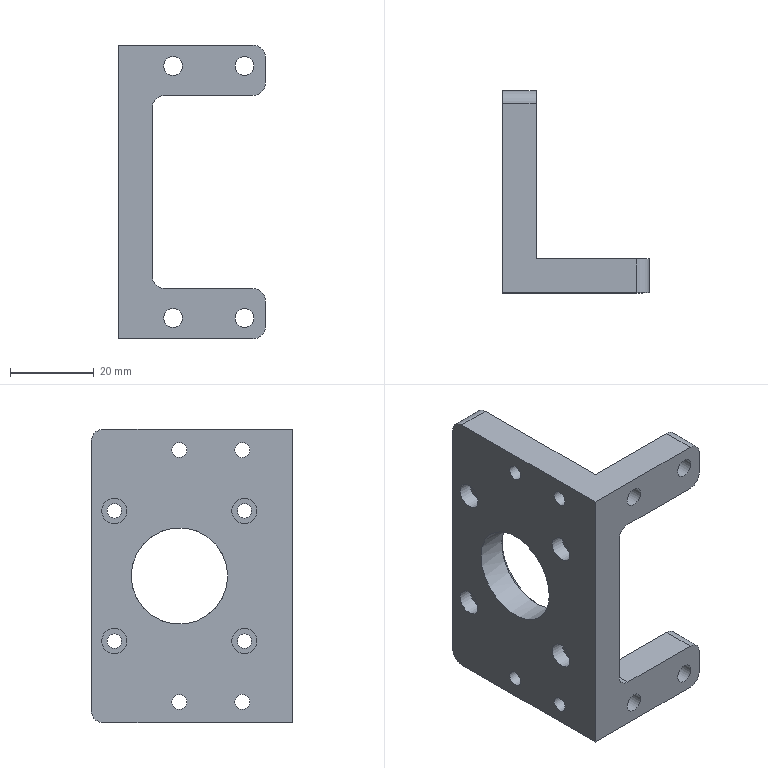Part | 1 solid | 58 faces | box 35 x 48 x 70 mm | volume 26377 mm3 | cylinder 33 | plane 24 | cone 1 | commonest cylinder face diameters 6 x16 3.4 x4 3.6 x4 4.5 x4 8 x4 23 x1
STEP:
#1=CARTESIAN_POINT('',(4.6,12.,68.));
#2=VERTEX_POINT('',#1);
#3=CARTESIAN_POINT('',(4.6,12.,65.));
#4=DIRECTION('',(1.,0.,0.));
#5=DIRECTION('',(0.,0.,1.));
#6=AXIS2_PLACEMENT_3D('',#3,#4,#5);
#7=CIRCLE('',#6,3.);
#8=EDGE_CURVE('',#2,#2,#7,.T.);
#9=ORIENTED_EDGE('',*,*,#8,.T.);
#10=EDGE_LOOP('',(#9));
#11=FACE_BOUND('',#10,.T.);
#12=CARTESIAN_POINT('',(4.6,12.,66.8));
#13=VERTEX_POINT('',#12);
#14=CARTESIAN_POINT('',(4.6,12.,65.));
#15=DIRECTION('',(1.,0.,0.));
#16=DIRECTION('',(0.,0.,1.));
#17=AXIS2_PLACEMENT_3D('',#14,#15,#16);
#18=CIRCLE('',#17,1.8);
#19=EDGE_CURVE('',#13,#13,#18,.T.);
#20=ORIENTED_EDGE('',*,*,#19,.F.);
#21=EDGE_LOOP('',(#20));
#22=FACE_BOUND('',#21,.T.);
#23=CARTESIAN_POINT('',(4.6,13.8,5.));
#24=DIRECTION('',(-1.,0.,0.));
#25=DIRECTION('',(0.,0.,1.));
#26=AXIS2_PLACEMENT_3D('',#23,#24,#25);
#27=PLANE('',#26);
#28=ADVANCED_FACE('',(#11,#22),#27,.F.);
#29=CARTESIAN_POINT('',(4.6,12.,2.));
#30=VERTEX_POINT('',#29);
#31=CARTESIAN_POINT('',(4.6,12.,5.));
#32=DIRECTION('',(1.,0.,0.));
#33=DIRECTION('',(0.,0.,-1.));
#34=AXIS2_PLACEMENT_3D('',#31,#32,#33);
#35=CIRCLE('',#34,3.);
#36=EDGE_CURVE('',#30,#30,#35,.T.);
#37=ORIENTED_EDGE('',*,*,#36,.T.);
#38=EDGE_LOOP('',(#37));
#39=FACE_BOUND('',#38,.T.);
#40=CARTESIAN_POINT('',(4.6,12.,3.2));
#41=VERTEX_POINT('',#40);
#42=CARTESIAN_POINT('',(4.6,12.,5.));
#43=DIRECTION('',(1.,0.,0.));
#44=DIRECTION('',(0.,0.,-1.));
#45=AXIS2_PLACEMENT_3D('',#42,#43,#44);
#46=CIRCLE('',#45,1.8);
#47=EDGE_CURVE('',#41,#41,#46,.T.);
#48=ORIENTED_EDGE('',*,*,#47,.F.);
#49=EDGE_LOOP('',(#48));
#50=FACE_BOUND('',#49,.T.);
#51=CARTESIAN_POINT('',(4.6,13.8,5.));
#52=DIRECTION('',(-1.,0.,0.));
#53=DIRECTION('',(0.,0.,1.));
#54=AXIS2_PLACEMENT_3D('',#51,#52,#53);
#55=PLANE('',#54);
#56=ADVANCED_FACE('',(#39,#50),#55,.F.);
#57=CARTESIAN_POINT('',(4.6,27.,68.));
#58=VERTEX_POINT('',#57);
#59=CARTESIAN_POINT('',(4.6,27.,65.));
#60=DIRECTION('',(1.,0.,0.));
#61=DIRECTION('',(0.,0.,1.));
#62=AXIS2_PLACEMENT_3D('',#59,#60,#61);
#63=CIRCLE('',#62,3.);
#64=EDGE_CURVE('',#58,#58,#63,.T.);
#65=ORIENTED_EDGE('',*,*,#64,.T.);
#66=EDGE_LOOP('',(#65));
#67=FACE_BOUND('',#66,.T.);
#68=CARTESIAN_POINT('',(4.6,27.,66.8));
#69=VERTEX_POINT('',#68);
#70=CARTESIAN_POINT('',(4.6,27.,65.));
#71=DIRECTION('',(1.,0.,0.));
#72=DIRECTION('',(0.,0.,1.));
#73=AXIS2_PLACEMENT_3D('',#70,#71,#72);
#74=CIRCLE('',#73,1.8);
#75=EDGE_CURVE('',#69,#69,#74,.T.);
#76=ORIENTED_EDGE('',*,*,#75,.F.);
#77=EDGE_LOOP('',(#76));
#78=FACE_BOUND('',#77,.T.);
#79=CARTESIAN_POINT('',(4.6,13.8,5.));
#80=DIRECTION('',(-1.,0.,0.));
#81=DIRECTION('',(0.,0.,1.));
#82=AXIS2_PLACEMENT_3D('',#79,#80,#81);
#83=PLANE('',#82);
#84=ADVANCED_FACE('',(#67,#78),#83,.F.);
#85=CARTESIAN_POINT('',(4.6,27.,8.));
#86=VERTEX_POINT('',#85);
#87=CARTESIAN_POINT('',(4.6,27.,5.));
#88=DIRECTION('',(1.,0.,0.));
#89=DIRECTION('',(0.,0.,1.));
#90=AXIS2_PLACEMENT_3D('',#87,#88,#89);
#91=CIRCLE('',#90,3.);
#92=EDGE_CURVE('',#86,#86,#91,.T.);
#93=ORIENTED_EDGE('',*,*,#92,.T.);
#94=EDGE_LOOP('',(#93));
#95=FACE_BOUND('',#94,.T.);
#96=CARTESIAN_POINT('',(4.6,27.,6.8));
#97=VERTEX_POINT('',#96);
#98=CARTESIAN_POINT('',(4.6,27.,5.));
#99=DIRECTION('',(1.,0.,0.));
#100=DIRECTION('',(0.,0.,1.));
#101=AXIS2_PLACEMENT_3D('',#98,#99,#100);
#102=CIRCLE('',#101,1.8);
#103=EDGE_CURVE('',#97,#97,#102,.T.);
#104=ORIENTED_EDGE('',*,*,#103,.F.);
#105=EDGE_LOOP('',(#104));
#106=FACE_BOUND('',#105,.T.);
#107=CARTESIAN_POINT('',(4.6,13.8,5.));
#108=DIRECTION('',(-1.,0.,0.));
#109=DIRECTION('',(0.,0.,1.));
#110=AXIS2_PLACEMENT_3D('',#107,#108,#109);
#111=PLANE('',#110);
#112=ADVANCED_FACE('',(#95,#106),#111,.F.);
#113=CARTESIAN_POINT('',(13.,3.4,69.));
#114=VERTEX_POINT('',#113);
#115=CARTESIAN_POINT('',(13.,3.4,65.));
#116=DIRECTION('',(0.,1.,0.));
#117=DIRECTION('',(0.,0.,1.));
#118=AXIS2_PLACEMENT_3D('',#115,#116,#117);
#119=CIRCLE('',#118,4.);
#120=EDGE_CURVE('',#114,#114,#119,.T.);
#121=ORIENTED_EDGE('',*,*,#120,.T.);
#122=EDGE_LOOP('',(#121));
#123=FACE_BOUND('',#122,.T.);
#124=CARTESIAN_POINT('',(13.,3.4,67.25));
#125=VERTEX_POINT('',#124);
#126=CARTESIAN_POINT('',(13.,3.4,65.));
#127=DIRECTION('',(0.,1.,0.));
#128=DIRECTION('',(0.,0.,1.));
#129=AXIS2_PLACEMENT_3D('',#126,#127,#128);
#130=CIRCLE('',#129,2.25);
#131=EDGE_CURVE('',#125,#125,#130,.T.);
#132=ORIENTED_EDGE('',*,*,#131,.F.);
#133=EDGE_LOOP('',(#132));
#134=FACE_BOUND('',#133,.T.);
#135=CARTESIAN_POINT('',(15.25,3.4,65.));
#136=DIRECTION('',(0.,-1.,0.));
#137=DIRECTION('',(0.,0.,-1.));
#138=AXIS2_PLACEMENT_3D('',#135,#136,#137);
#139=PLANE('',#138);
#140=ADVANCED_FACE('',(#123,#134),#139,.F.);
#141=CARTESIAN_POINT('',(30.,3.4,61.));
#142=VERTEX_POINT('',#141);
#143=CARTESIAN_POINT('',(30.,3.4,65.));
#144=DIRECTION('',(0.,1.,0.));
#145=DIRECTION('',(0.,0.,-1.));
#146=AXIS2_PLACEMENT_3D('',#143,#144,#145);
#147=CIRCLE('',#146,4.);
#148=EDGE_CURVE('',#142,#142,#147,.T.);
#149=ORIENTED_EDGE('',*,*,#148,.T.);
#150=EDGE_LOOP('',(#149));
#151=FACE_BOUND('',#150,.T.);
#152=CARTESIAN_POINT('',(30.,3.4,62.75));
#153=VERTEX_POINT('',#152);
#154=CARTESIAN_POINT('',(30.,3.4,65.));
#155=DIRECTION('',(0.,1.,0.));
#156=DIRECTION('',(0.,0.,-1.));
#157=AXIS2_PLACEMENT_3D('',#154,#155,#156);
#158=CIRCLE('',#157,2.25);
#159=EDGE_CURVE('',#153,#153,#158,.T.);
#160=ORIENTED_EDGE('',*,*,#159,.F.);
#161=EDGE_LOOP('',(#160));
#162=FACE_BOUND('',#161,.T.);
#163=CARTESIAN_POINT('',(15.25,3.4,65.));
#164=DIRECTION('',(0.,-1.,0.));
#165=DIRECTION('',(0.,0.,-1.));
#166=AXIS2_PLACEMENT_3D('',#163,#164,#165);
#167=PLANE('',#166);
#168=ADVANCED_FACE('',(#151,#162),#167,.F.);
#169=CARTESIAN_POINT('',(13.,3.4,1.));
#170=VERTEX_POINT('',#169);
#171=CARTESIAN_POINT('',(13.,3.4,5.));
#172=DIRECTION('',(0.,1.,0.));
#173=DIRECTION('',(0.,0.,-1.));
#174=AXIS2_PLACEMENT_3D('',#171,#172,#173);
#175=CIRCLE('',#174,4.);
#176=EDGE_CURVE('',#170,#170,#175,.T.);
#177=ORIENTED_EDGE('',*,*,#176,.T.);
#178=EDGE_LOOP('',(#177));
#179=FACE_BOUND('',#178,.T.);
#180=CARTESIAN_POINT('',(13.,3.4,2.75));
#181=VERTEX_POINT('',#180);
#182=CARTESIAN_POINT('',(13.,3.4,5.));
#183=DIRECTION('',(0.,1.,0.));
#184=DIRECTION('',(0.,0.,-1.));
#185=AXIS2_PLACEMENT_3D('',#182,#183,#184);
#186=CIRCLE('',#185,2.25);
#187=EDGE_CURVE('',#181,#181,#186,.T.);
#188=ORIENTED_EDGE('',*,*,#187,.F.);
#189=EDGE_LOOP('',(#188));
#190=FACE_BOUND('',#189,.T.);
#191=CARTESIAN_POINT('',(15.25,3.4,65.));
#192=DIRECTION('',(0.,-1.,0.));
#193=DIRECTION('',(0.,0.,-1.));
#194=AXIS2_PLACEMENT_3D('',#191,#192,#193);
#195=PLANE('',#194);
#196=ADVANCED_FACE('',(#179,#190),#195,.F.);
#197=CARTESIAN_POINT('',(30.,3.4,1.));
#198=VERTEX_POINT('',#197);
#199=CARTESIAN_POINT('',(30.,3.4,5.));
#200=DIRECTION('',(0.,1.,0.));
#201=DIRECTION('',(0.,0.,-1.));
#202=AXIS2_PLACEMENT_3D('',#199,#200,#201);
#203=CIRCLE('',#202,4.);
#204=EDGE_CURVE('',#198,#198,#203,.T.);
#205=ORIENTED_EDGE('',*,*,#204,.T.);
#206=EDGE_LOOP('',(#205));
#207=FACE_BOUND('',#206,.T.);
#208=CARTESIAN_POINT('',(30.,3.4,2.75));
#209=VERTEX_POINT('',#208);
#210=CARTESIAN_POINT('',(30.,3.4,5.));
#211=DIRECTION('',(0.,1.,0.));
#212=DIRECTION('',(0.,0.,-1.));
#213=AXIS2_PLACEMENT_3D('',#210,#211,#212);
#214=CIRCLE('',#213,2.25);
#215=EDGE_CURVE('',#209,#209,#214,.T.);
#216=ORIENTED_EDGE('',*,*,#215,.F.);
#217=EDGE_LOOP('',(#216));
#218=FACE_BOUND('',#217,.T.);
#219=CARTESIAN_POINT('',(15.25,3.4,65.));
#220=DIRECTION('',(0.,-1.,0.));
#221=DIRECTION('',(0.,0.,-1.));
#222=AXIS2_PLACEMENT_3D('',#219,#220,#221);
#223=PLANE('',#222);
#224=ADVANCED_FACE('',(#207,#218),#223,.F.);
#225=CARTESIAN_POINT('',(8.,0.,55.));
#226=VERTEX_POINT('',#225);
#227=CARTESIAN_POINT('',(11.,0.,58.));
#228=VERTEX_POINT('',#227);
#229=CARTESIAN_POINT('',(11.,0.,55.));
#230=DIRECTION('',(0.,1.,0.));
#231=DIRECTION('',(0.,0.,1.));
#232=AXIS2_PLACEMENT_3D('',#229,#230,#231);
#233=CIRCLE('',#232,3.);
#234=EDGE_CURVE('',#226,#228,#233,.T.);
#235=ORIENTED_EDGE('',*,*,#234,.F.);
#236=CARTESIAN_POINT('',(8.,8.,55.));
#237=VERTEX_POINT('',#236);
#238=CARTESIAN_POINT('',(8.,0.,55.));
#239=DIRECTION('',(0.,-1.,0.));
#240=VECTOR('',#239,1000.);
#241=LINE('',#238,#240);
#242=EDGE_CURVE('',#237,#226,#241,.T.);
#243=ORIENTED_EDGE('',*,*,#242,.F.);
#244=CARTESIAN_POINT('',(11.,8.,58.));
#245=VERTEX_POINT('',#244);
#246=CARTESIAN_POINT('',(11.,8.,55.));
#247=DIRECTION('',(0.,-1.,0.));
#248=DIRECTION('',(1.,0.,0.));
#249=AXIS2_PLACEMENT_3D('',#246,#247,#248);
#250=CIRCLE('',#249,3.);
#251=EDGE_CURVE('',#245,#237,#250,.T.);
#252=ORIENTED_EDGE('',*,*,#251,.F.);
#253=CARTESIAN_POINT('',(11.,8.,58.));
#254=DIRECTION('',(0.,1.,0.));
#255=VECTOR('',#254,1000.);
#256=LINE('',#253,#255);
#257=EDGE_CURVE('',#228,#245,#256,.T.);
#258=ORIENTED_EDGE('',*,*,#257,.F.);
#259=EDGE_LOOP('',(#235,#243,#252,#258));
#260=FACE_BOUND('',#259,.T.);
#261=CARTESIAN_POINT('',(11.,-2.,55.));
#262=DIRECTION('',(0.,-1.,0.));
#263=DIRECTION('',(0.,0.,-1.));
#264=AXIS2_PLACEMENT_3D('',#261,#262,#263);
#265=CYLINDRICAL_SURFACE('',#264,3.);
#266=ADVANCED_FACE('',(#260),#265,.F.);
#267=CARTESIAN_POINT('',(11.,0.,12.));
#268=VERTEX_POINT('',#267);
#269=CARTESIAN_POINT('',(8.,0.,15.));
#270=VERTEX_POINT('',#269);
#271=CARTESIAN_POINT('',(11.,0.,15.));
#272=DIRECTION('',(0.,1.,0.));
#273=DIRECTION('',(0.,0.,1.));
#274=AXIS2_PLACEMENT_3D('',#271,#272,#273);
#275=CIRCLE('',#274,3.);
#276=EDGE_CURVE('',#268,#270,#275,.T.);
#277=ORIENTED_EDGE('',*,*,#276,.F.);
#278=CARTESIAN_POINT('',(11.,8.,12.));
#279=VERTEX_POINT('',#278);
#280=CARTESIAN_POINT('',(11.,0.,12.));
#281=DIRECTION('',(0.,-1.,0.));
#282=VECTOR('',#281,1000.);
#283=LINE('',#280,#282);
#284=EDGE_CURVE('',#279,#268,#283,.T.);
#285=ORIENTED_EDGE('',*,*,#284,.F.);
#286=CARTESIAN_POINT('',(8.,8.,15.));
#287=VERTEX_POINT('',#286);
#288=CARTESIAN_POINT('',(11.,8.,15.));
#289=DIRECTION('',(0.,-1.,0.));
#290=DIRECTION('',(1.,0.,0.));
#291=AXIS2_PLACEMENT_3D('',#288,#289,#290);
#292=CIRCLE('',#291,3.);
#293=EDGE_CURVE('',#287,#279,#292,.T.);
#294=ORIENTED_EDGE('',*,*,#293,.F.);
#295=CARTESIAN_POINT('',(8.,8.,15.));
#296=DIRECTION('',(0.,1.,0.));
#297=VECTOR('',#296,1000.);
#298=LINE('',#295,#297);
#299=EDGE_CURVE('',#270,#287,#298,.T.);
#300=ORIENTED_EDGE('',*,*,#299,.F.);
#301=EDGE_LOOP('',(#277,#285,#294,#300));
#302=FACE_BOUND('',#301,.T.);
#303=CARTESIAN_POINT('',(11.,8.,15.));
#304=DIRECTION('',(0.,-1.,0.));
#305=DIRECTION('',(0.,0.,-1.));
#306=AXIS2_PLACEMENT_3D('',#303,#304,#305);
#307=CYLINDRICAL_SURFACE('',#306,3.);
#308=ADVANCED_FACE('',(#302),#307,.F.);
#309=CARTESIAN_POINT('',(35.,0.,9.));
#310=VERTEX_POINT('',#309);
#311=CARTESIAN_POINT('',(32.,0.,12.));
#312=VERTEX_POINT('',#311);
#313=CARTESIAN_POINT('',(32.,0.,9.));
#314=DIRECTION('',(0.,-1.,0.));
#315=DIRECTION('',(0.,0.,1.));
#316=AXIS2_PLACEMENT_3D('',#313,#314,#315);
#317=CIRCLE('',#316,3.);
#318=EDGE_CURVE('',#310,#312,#317,.T.);
#319=ORIENTED_EDGE('',*,*,#318,.F.);
#320=CARTESIAN_POINT('',(35.,8.,9.));
#321=VERTEX_POINT('',#320);
#322=CARTESIAN_POINT('',(35.,0.,9.));
#323=DIRECTION('',(0.,-1.,0.));
#324=VECTOR('',#323,1000.);
#325=LINE('',#322,#324);
#326=EDGE_CURVE('',#321,#310,#325,.T.);
#327=ORIENTED_EDGE('',*,*,#326,.F.);
#328=CARTESIAN_POINT('',(32.,8.,12.));
#329=VERTEX_POINT('',#328);
#330=CARTESIAN_POINT('',(32.,8.,9.));
#331=DIRECTION('',(0.,1.,0.));
#332=DIRECTION('',(1.,0.,0.));
#333=AXIS2_PLACEMENT_3D('',#330,#331,#332);
#334=CIRCLE('',#333,3.);
#335=EDGE_CURVE('',#329,#321,#334,.T.);
#336=ORIENTED_EDGE('',*,*,#335,.F.);
#337=CARTESIAN_POINT('',(32.,-2.,12.));
#338=DIRECTION('',(0.,1.,0.));
#339=VECTOR('',#338,1000.);
#340=LINE('',#337,#339);
#341=EDGE_CURVE('',#312,#329,#340,.T.);
#342=ORIENTED_EDGE('',*,*,#341,.F.);
#343=EDGE_LOOP('',(#319,#327,#336,#342));
#344=FACE_BOUND('',#343,.T.);
#345=CARTESIAN_POINT('',(32.,-2.,9.));
#346=DIRECTION('',(0.,1.,0.));
#347=DIRECTION('',(0.,0.,1.));
#348=AXIS2_PLACEMENT_3D('',#345,#346,#347);
#349=CYLINDRICAL_SURFACE('',#348,3.);
#350=ADVANCED_FACE('',(#344),#349,.T.);
#351=CARTESIAN_POINT('',(32.,0.,0.));
#352=VERTEX_POINT('',#351);
#353=CARTESIAN_POINT('',(35.,0.,3.));
#354=VERTEX_POINT('',#353);
#355=CARTESIAN_POINT('',(32.,0.,3.));
#356=DIRECTION('',(0.,-1.,0.));
#357=DIRECTION('',(0.,0.,1.));
#358=AXIS2_PLACEMENT_3D('',#355,#356,#357);
#359=CIRCLE('',#358,3.);
#360=EDGE_CURVE('',#352,#354,#359,.T.);
#361=ORIENTED_EDGE('',*,*,#360,.F.);
#362=CARTESIAN_POINT('',(32.,8.,0.));
#363=VERTEX_POINT('',#362);
#364=CARTESIAN_POINT('',(32.,0.,0.));
#365=DIRECTION('',(0.,-1.,0.));
#366=VECTOR('',#365,1000.);
#367=LINE('',#364,#366);
#368=EDGE_CURVE('',#363,#352,#367,.T.);
#369=ORIENTED_EDGE('',*,*,#368,.F.);
#370=CARTESIAN_POINT('',(35.,8.,3.));
#371=VERTEX_POINT('',#370);
#372=CARTESIAN_POINT('',(32.,8.,3.));
#373=DIRECTION('',(0.,1.,0.));
#374=DIRECTION('',(1.,0.,0.));
#375=AXIS2_PLACEMENT_3D('',#372,#373,#374);
#376=CIRCLE('',#375,3.);
#377=EDGE_CURVE('',#371,#363,#376,.T.);
#378=ORIENTED_EDGE('',*,*,#377,.F.);
#379=CARTESIAN_POINT('',(35.,0.,3.));
#380=DIRECTION('',(0.,1.,0.));
#381=VECTOR('',#380,1000.);
#382=LINE('',#379,#381);
#383=EDGE_CURVE('',#354,#371,#382,.T.);
#384=ORIENTED_EDGE('',*,*,#383,.F.);
#385=EDGE_LOOP('',(#361,#369,#378,#384));
#386=FACE_BOUND('',#385,.T.);
#387=CARTESIAN_POINT('',(32.,0.,3.));
#388=DIRECTION('',(0.,1.,0.));
#389=DIRECTION('',(0.,0.,1.));
#390=AXIS2_PLACEMENT_3D('',#387,#388,#389);
#391=CYLINDRICAL_SURFACE('',#390,3.);
#392=ADVANCED_FACE('',(#386),#391,.T.);
#393=CARTESIAN_POINT('',(32.,0.,58.));
#394=VERTEX_POINT('',#393);
#395=CARTESIAN_POINT('',(35.,0.,61.));
#396=VERTEX_POINT('',#395);
#397=CARTESIAN_POINT('',(32.,0.,61.));
#398=DIRECTION('',(0.,-1.,0.));
#399=DIRECTION('',(0.,0.,1.));
#400=AXIS2_PLACEMENT_3D('',#397,#398,#399);
#401=CIRCLE('',#400,3.);
#402=EDGE_CURVE('',#394,#396,#401,.T.);
#403=ORIENTED_EDGE('',*,*,#402,.F.);
#404=CARTESIAN_POINT('',(32.,8.,58.));
#405=VERTEX_POINT('',#404);
#406=CARTESIAN_POINT('',(32.,-2.,58.));
#407=DIRECTION('',(0.,-1.,0.));
#408=VECTOR('',#407,1000.);
#409=LINE('',#406,#408);
#410=EDGE_CURVE('',#405,#394,#409,.T.);
#411=ORIENTED_EDGE('',*,*,#410,.F.);
#412=CARTESIAN_POINT('',(35.,8.,61.));
#413=VERTEX_POINT('',#412);
#414=CARTESIAN_POINT('',(32.,8.,61.));
#415=DIRECTION('',(0.,1.,0.));
#416=DIRECTION('',(1.,0.,0.));
#417=AXIS2_PLACEMENT_3D('',#414,#415,#416);
#418=CIRCLE('',#417,3.);
#419=EDGE_CURVE('',#413,#405,#418,.T.);
#420=ORIENTED_EDGE('',*,*,#419,.F.);
#421=CARTESIAN_POINT('',(35.,0.,61.));
#422=DIRECTION('',(0.,1.,0.));
#423=VECTOR('',#422,1000.);
#424=LINE('',#421,#423);
#425=EDGE_CURVE('',#396,#413,#424,.T.);
#426=ORIENTED_EDGE('',*,*,#425,.F.);
#427=EDGE_LOOP('',(#403,#411,#420,#426));
#428=FACE_BOUND('',#427,.T.);
#429=CARTESIAN_POINT('',(32.,0.,61.));
#430=DIRECTION('',(0.,1.,0.));
#431=DIRECTION('',(0.,0.,1.));
#432=AXIS2_PLACEMENT_3D('',#429,#430,#431);
#433=CYLINDRICAL_SURFACE('',#432,3.);
#434=ADVANCED_FACE('',(#428),#433,.T.);
#435=CARTESIAN_POINT('',(35.,0.,67.));
#436=VERTEX_POINT('',#435);
#437=CARTESIAN_POINT('',(32.,0.,70.));
#438=VERTEX_POINT('',#437);
#439=CARTESIAN_POINT('',(32.,0.,67.));
#440=DIRECTION('',(0.,-1.,0.));
#441=DIRECTION('',(0.,0.,1.));
#442=AXIS2_PLACEMENT_3D('',#439,#440,#441);
#443=CIRCLE('',#442,3.);
#444=EDGE_CURVE('',#436,#438,#443,.T.);
#445=ORIENTED_EDGE('',*,*,#444,.F.);
#446=CARTESIAN_POINT('',(35.,8.,67.));
#447=VERTEX_POINT('',#446);
#448=CARTESIAN_POINT('',(35.,0.,67.));
#449=DIRECTION('',(0.,-1.,0.));
#450=VECTOR('',#449,1000.);
#451=LINE('',#448,#450);
#452=EDGE_CURVE('',#447,#436,#451,.T.);
#453=ORIENTED_EDGE('',*,*,#452,.F.);
#454=CARTESIAN_POINT('',(32.,8.,70.));
#455=VERTEX_POINT('',#454);
#456=CARTESIAN_POINT('',(32.,8.,67.));
#457=DIRECTION('',(0.,1.,0.));
#458=DIRECTION('',(1.,0.,0.));
#459=AXIS2_PLACEMENT_3D('',#456,#457,#458);
#460=CIRCLE('',#459,3.);
#461=EDGE_CURVE('',#455,#447,#460,.T.);
#462=ORIENTED_EDGE('',*,*,#461,.F.);
#463=CARTESIAN_POINT('',(32.,8.,70.));
#464=DIRECTION('',(0.,1.,0.));
#465=VECTOR('',#464,1000.);
#466=LINE('',#463,#465);
#467=EDGE_CURVE('',#438,#455,#466,.T.);
#468=ORIENTED_EDGE('',*,*,#467,.F.);
#469=EDGE_LOOP('',(#445,#453,#462,#468));
#470=FACE_BOUND('',#469,.T.);
#471=CARTESIAN_POINT('',(32.,0.,67.));
#472=DIRECTION('',(0.,-1.,0.));
#473=DIRECTION('',(0.,0.,-1.));
#474=AXIS2_PLACEMENT_3D('',#471,#472,#473);
#475=CYLINDRICAL_SURFACE('',#474,3.);
#476=ADVANCED_FACE('',(#470),#475,.T.);
#477=CARTESIAN_POINT('',(8.,48.,67.));
#478=VERTEX_POINT('',#477);
#479=CARTESIAN_POINT('',(8.,45.,70.));
#480=VERTEX_POINT('',#479);
#481=CARTESIAN_POINT('',(8.,45.,67.));
#482=DIRECTION('',(1.,0.,0.));
#483=DIRECTION('',(0.,0.,1.));
#484=AXIS2_PLACEMENT_3D('',#481,#482,#483);
#485=CIRCLE('',#484,3.);
#486=EDGE_CURVE('',#478,#480,#485,.T.);
#487=ORIENTED_EDGE('',*,*,#486,.F.);
#488=CARTESIAN_POINT('',(0.,48.,67.));
#489=VERTEX_POINT('',#488);
#490=CARTESIAN_POINT('',(8.,48.,67.));
#491=DIRECTION('',(1.,0.,0.));
#492=VECTOR('',#491,1000.);
#493=LINE('',#490,#492);
#494=EDGE_CURVE('',#489,#478,#493,.T.);
#495=ORIENTED_EDGE('',*,*,#494,.F.);
#496=CARTESIAN_POINT('',(0.,45.,70.));
#497=VERTEX_POINT('',#496);
#498=CARTESIAN_POINT('',(0.,45.,67.));
#499=DIRECTION('',(-1.,0.,0.));
#500=DIRECTION('',(0.,0.,-1.));
#501=AXIS2_PLACEMENT_3D('',#498,#499,#500);
#502=CIRCLE('',#501,3.);
#503=EDGE_CURVE('',#497,#489,#502,.T.);
#504=ORIENTED_EDGE('',*,*,#503,.F.);
#505=CARTESIAN_POINT('',(0.,45.,70.));
#506=DIRECTION('',(-1.,0.,0.));
#507=VECTOR('',#506,1000.);
#508=LINE('',#505,#507);
#509=EDGE_CURVE('',#480,#497,#508,.T.);
#510=ORIENTED_EDGE('',*,*,#509,.F.);
#511=EDGE_LOOP('',(#487,#495,#504,#510));
#512=FACE_BOUND('',#511,.T.);
#513=CARTESIAN_POINT('',(0.,45.,67.));
#514=DIRECTION('',(1.,0.,0.));
#515=DIRECTION('',(0.,0.,-1.));
#516=AXIS2_PLACEMENT_3D('',#513,#514,#515);
#517=CYLINDRICAL_SURFACE('',#516,3.);
#518=ADVANCED_FACE('',(#512),#517,.T.);
#519=CARTESIAN_POINT('',(8.,45.,0.));
#520=VERTEX_POINT('',#519);
#521=CARTESIAN_POINT('',(8.,48.,3.));
#522=VERTEX_POINT('',#521);
#523=CARTESIAN_POINT('',(8.,45.,3.));
#524=DIRECTION('',(1.,0.,0.));
#525=DIRECTION('',(0.,0.,1.));
#526=AXIS2_PLACEMENT_3D('',#523,#524,#525);
#527=CIRCLE('',#526,3.);
#528=EDGE_CURVE('',#520,#522,#527,.T.);
#529=ORIENTED_EDGE('',*,*,#528,.F.);
#530=CARTESIAN_POINT('',(0.,45.,0.));
#531=VERTEX_POINT('',#530);
#532=CARTESIAN_POINT('',(0.,45.,0.));
#533=DIRECTION('',(1.,0.,0.));
#534=VECTOR('',#533,1000.);
#535=LINE('',#532,#534);
#536=EDGE_CURVE('',#531,#520,#535,.T.);
#537=ORIENTED_EDGE('',*,*,#536,.F.);
#538=CARTESIAN_POINT('',(0.,48.,3.));
#539=VERTEX_POINT('',#538);
#540=CARTESIAN_POINT('',(0.,45.,3.));
#541=DIRECTION('',(-1.,0.,0.));
#542=DIRECTION('',(0.,0.,-1.));
#543=AXIS2_PLACEMENT_3D('',#540,#541,#542);
#544=CIRCLE('',#543,3.);
#545=EDGE_CURVE('',#539,#531,#544,.T.);
#546=ORIENTED_EDGE('',*,*,#545,.F.);
#547=CARTESIAN_POINT('',(8.,48.,3.));
#548=DIRECTION('',(-1.,0.,0.));
#549=VECTOR('',#548,1000.);
#550=LINE('',#547,#549);
#551=EDGE_CURVE('',#522,#539,#550,.T.);
#552=ORIENTED_EDGE('',*,*,#551,.F.);
#553=EDGE_LOOP('',(#529,#537,#546,#552));
#554=FACE_BOUND('',#553,.T.);
#555=CARTESIAN_POINT('',(8.,45.,3.));
#556=DIRECTION('',(-1.,0.,0.));
#557=DIRECTION('',(0.,0.,1.));
#558=AXIS2_PLACEMENT_3D('',#555,#556,#557);
#559=CYLINDRICAL_SURFACE('',#558,3.);
#560=ADVANCED_FACE('',(#554),#559,.T.);
#561=CARTESIAN_POINT('',(8.,8.,58.));
#562=DIRECTION('',(1.,0.,0.));
#563=VECTOR('',#562,1000.);
#564=LINE('',#561,#563);
#565=EDGE_CURVE('',#245,#405,#564,.T.);
#566=ORIENTED_EDGE('',*,*,#565,.T.);
#567=ORIENTED_EDGE('',*,*,#410,.T.);
#568=CARTESIAN_POINT('',(0.,0.,58.));
#569=DIRECTION('',(1.,0.,0.));
#570=VECTOR('',#569,1000.);
#571=LINE('',#568,#570);
#572=EDGE_CURVE('',#228,#394,#571,.T.);
#573=ORIENTED_EDGE('',*,*,#572,.F.);
#574=ORIENTED_EDGE('',*,*,#257,.T.);
#575=EDGE_LOOP('',(#566,#567,#573,#574));
#576=FACE_BOUND('',#575,.T.);
#577=CARTESIAN_POINT('',(8.,-2.,58.));
#578=DIRECTION('',(0.,0.,1.));
#579=DIRECTION('',(1.,0.,0.));
#580=AXIS2_PLACEMENT_3D('',#577,#578,#579);
#581=PLANE('',#580);
#582=ADVANCED_FACE('',(#576),#581,.F.);
#583=CARTESIAN_POINT('',(0.,0.,12.));
#584=DIRECTION('',(-1.,0.,0.));
#585=VECTOR('',#584,1000.);
#586=LINE('',#583,#585);
#587=EDGE_CURVE('',#312,#268,#586,.T.);
#588=ORIENTED_EDGE('',*,*,#587,.F.);
#589=ORIENTED_EDGE('',*,*,#341,.T.);
#590=CARTESIAN_POINT('',(8.,8.,12.));
#591=DIRECTION('',(-1.,0.,0.));
#592=VECTOR('',#591,1000.);
#593=LINE('',#590,#592);
#594=EDGE_CURVE('',#329,#279,#593,.T.);
#595=ORIENTED_EDGE('',*,*,#594,.T.);
#596=ORIENTED_EDGE('',*,*,#284,.T.);
#597=EDGE_LOOP('',(#588,#589,#595,#596));
#598=FACE_BOUND('',#597,.T.);
#599=CARTESIAN_POINT('',(8.,-2.,12.));
#600=DIRECTION('',(0.,0.,-1.));
#601=DIRECTION('',(-1.,0.,0.));
#602=AXIS2_PLACEMENT_3D('',#599,#600,#601);
#603=PLANE('',#602);
#604=ADVANCED_FACE('',(#598),#603,.F.);
#605=CARTESIAN_POINT('',(3.4,42.5,53.5));
#606=VERTEX_POINT('',#605);
#607=CARTESIAN_POINT('',(3.4,42.5,50.5));
#608=DIRECTION('',(-1.,0.,0.));
#609=DIRECTION('',(0.,0.,1.));
#610=AXIS2_PLACEMENT_3D('',#607,#608,#609);
#611=CIRCLE('',#610,3.);
#612=EDGE_CURVE('',#606,#606,#611,.T.);
#613=ORIENTED_EDGE('',*,*,#612,.T.);
#614=EDGE_LOOP('',(#613));
#615=FACE_BOUND('',#614,.T.);
#616=CARTESIAN_POINT('',(3.4,42.5,52.2));
#617=VERTEX_POINT('',#616);
#618=CARTESIAN_POINT('',(3.4,42.5,50.5));
#619=DIRECTION('',(-1.,0.,0.));
#620=DIRECTION('',(0.,0.,1.));
#621=AXIS2_PLACEMENT_3D('',#618,#619,#620);
#622=CIRCLE('',#621,1.7);
#623=EDGE_CURVE('',#617,#617,#622,.T.);
#624=ORIENTED_EDGE('',*,*,#623,.F.);
#625=EDGE_LOOP('',(#624));
#626=FACE_BOUND('',#625,.T.);
#627=CARTESIAN_POINT('',(3.4,44.2,50.5));
#628=DIRECTION('',(1.,0.,0.));
#629=DIRECTION('',(0.,0.,-1.));
#630=AXIS2_PLACEMENT_3D('',#627,#628,#629);
#631=PLANE('',#630);
#632=ADVANCED_FACE('',(#615,#626),#631,.F.);
#633=CARTESIAN_POINT('',(3.4,11.5,16.5));
#634=VERTEX_POINT('',#633);
#635=CARTESIAN_POINT('',(3.4,11.5,19.5));
#636=DIRECTION('',(-1.,0.,0.));
#637=DIRECTION('',(0.,0.,-1.));
#638=AXIS2_PLACEMENT_3D('',#635,#636,#637);
#639=CIRCLE('',#638,3.);
#640=EDGE_CURVE('',#634,#634,#639,.T.);
#641=ORIENTED_EDGE('',*,*,#640,.T.);
#642=EDGE_LOOP('',(#641));
#643=FACE_BOUND('',#642,.T.);
#644=CARTESIAN_POINT('',(3.4,11.5,17.8));
#645=VERTEX_POINT('',#644);
#646=CARTESIAN_POINT('',(3.4,11.5,19.5));
#647=DIRECTION('',(-1.,0.,0.));
#648=DIRECTION('',(0.,0.,-1.));
#649=AXIS2_PLACEMENT_3D('',#646,#647,#648);
#650=CIRCLE('',#649,1.7);
#651=EDGE_CURVE('',#645,#645,#650,.T.);
#652=ORIENTED_EDGE('',*,*,#651,.F.);
#653=EDGE_LOOP('',(#652));
#654=FACE_BOUND('',#653,.T.);
#655=CARTESIAN_POINT('',(3.4,44.2,50.5));
#656=DIRECTION('',(1.,0.,0.));
#657=DIRECTION('',(0.,0.,-1.));
#658=AXIS2_PLACEMENT_3D('',#655,#656,#657);
#659=PLANE('',#658);
#660=ADVANCED_FACE('',(#643,#654),#659,.F.);
#661=CARTESIAN_POINT('',(3.4,42.5,16.5));
#662=VERTEX_POINT('',#661);
#663=CARTESIAN_POINT('',(3.4,42.5,19.5));
#664=DIRECTION('',(-1.,0.,0.));
#665=DIRECTION('',(0.,0.,-1.));
#666=AXIS2_PLACEMENT_3D('',#663,#664,#665);
#667=CIRCLE('',#666,3.);
#668=EDGE_CURVE('',#662,#662,#667,.T.);
#669=ORIENTED_EDGE('',*,*,#668,.T.);
#670=EDGE_LOOP('',(#669));
#671=FACE_BOUND('',#670,.T.);
#672=CARTESIAN_POINT('',(3.4,42.5,17.8));
#673=VERTEX_POINT('',#672);
#674=CARTESIAN_POINT('',(3.4,42.5,19.5));
#675=DIRECTION('',(-1.,0.,0.));
#676=DIRECTION('',(0.,0.,-1.));
#677=AXIS2_PLACEMENT_3D('',#674,#675,#676);
#678=CIRCLE('',#677,1.7);
#679=EDGE_CURVE('',#673,#673,#678,.T.);
#680=ORIENTED_EDGE('',*,*,#679,.F.);
#681=EDGE_LOOP('',(#680));
#682=FACE_BOUND('',#681,.T.);
#683=CARTESIAN_POINT('',(3.4,44.2,50.5));
#684=DIRECTION('',(1.,0.,0.));
#685=DIRECTION('',(0.,0.,-1.));
#686=AXIS2_PLACEMENT_3D('',#683,#684,#685);
#687=PLANE('',#686);
#688=ADVANCED_FACE('',(#671,#682),#687,.F.);
#689=CARTESIAN_POINT('',(3.4,11.5,47.5));
#690=VERTEX_POINT('',#689);
#691=CARTESIAN_POINT('',(3.4,11.5,50.5));
#692=DIRECTION('',(-1.,0.,0.));
#693=DIRECTION('',(0.,0.,-1.));
#694=AXIS2_PLACEMENT_3D('',#691,#692,#693);
#695=CIRCLE('',#694,3.);
#696=EDGE_CURVE('',#690,#690,#695,.T.);
#697=ORIENTED_EDGE('',*,*,#696,.T.);
#698=EDGE_LOOP('',(#697));
#699=FACE_BOUND('',#698,.T.);
#700=CARTESIAN_POINT('',(3.4,11.5,48.8));
#701=VERTEX_POINT('',#700);
#702=CARTESIAN_POINT('',(3.4,11.5,50.5));
#703=DIRECTION('',(-1.,0.,0.));
#704=DIRECTION('',(0.,0.,-1.));
#705=AXIS2_PLACEMENT_3D('',#702,#703,#704);
#706=CIRCLE('',#705,1.7);
#707=EDGE_CURVE('',#701,#701,#706,.T.);
#708=ORIENTED_EDGE('',*,*,#707,.F.);
#709=EDGE_LOOP('',(#708));
#710=FACE_BOUND('',#709,.T.);
#711=CARTESIAN_POINT('',(3.4,44.2,50.5));
#712=DIRECTION('',(1.,0.,0.));
#713=DIRECTION('',(0.,0.,-1.));
#714=AXIS2_PLACEMENT_3D('',#711,#712,#713);
#715=PLANE('',#714);
#716=ADVANCED_FACE('',(#699,#710),#715,.F.);
#717=CARTESIAN_POINT('',(0.,0.,0.));
#718=VERTEX_POINT('',#717);
#719=CARTESIAN_POINT('',(0.,48.,0.));
#720=DIRECTION('',(0.,-1.,0.));
#721=VECTOR('',#720,1000.);
#722=LINE('',#719,#721);
#723=EDGE_CURVE('',#531,#718,#722,.T.);
#724=ORIENTED_EDGE('',*,*,#723,.F.);
#725=ORIENTED_EDGE('',*,*,#536,.T.);
#726=CARTESIAN_POINT('',(8.,8.,0.));
#727=VERTEX_POINT('',#726);
#728=CARTESIAN_POINT('',(8.,8.,0.));
#729=DIRECTION('',(0.,1.,0.));
#730=VECTOR('',#729,1000.);
#731=LINE('',#728,#730);
#732=EDGE_CURVE('',#727,#520,#731,.T.);
#733=ORIENTED_EDGE('',*,*,#732,.F.);
#734=CARTESIAN_POINT('',(35.,8.,0.));
#735=DIRECTION('',(-1.,0.,0.));
#736=VECTOR('',#735,1000.);
#737=LINE('',#734,#736);
#738=EDGE_CURVE('',#363,#727,#737,.T.);
#739=ORIENTED_EDGE('',*,*,#738,.F.);
#740=ORIENTED_EDGE('',*,*,#368,.T.);
#741=CARTESIAN_POINT('',(0.,0.,0.));
#742=DIRECTION('',(1.,0.,0.));
#743=VECTOR('',#742,1000.);
#744=LINE('',#741,#743);
#745=EDGE_CURVE('',#718,#352,#744,.T.);
#746=ORIENTED_EDGE('',*,*,#745,.F.);
#747=EDGE_LOOP('',(#724,#725,#733,#739,#740,#746));
#748=FACE_BOUND('',#747,.T.);
#749=CARTESIAN_POINT('',(0.,0.,0.));
#750=DIRECTION('',(0.,0.,1.));
#751=DIRECTION('',(1.,0.,0.));
#752=AXIS2_PLACEMENT_3D('',#749,#750,#751);
#753=PLANE('',#752);
#754=ADVANCED_FACE('',(#748),#753,.F.);
#755=CARTESIAN_POINT('',(8.,8.,70.));
#756=VERTEX_POINT('',#755);
#757=CARTESIAN_POINT('',(8.,8.,70.));
#758=DIRECTION('',(0.,1.,0.));
#759=VECTOR('',#758,1000.);
#760=LINE('',#757,#759);
#761=EDGE_CURVE('',#756,#480,#760,.T.);
#762=ORIENTED_EDGE('',*,*,#761,.T.);
#763=ORIENTED_EDGE('',*,*,#509,.T.);
#764=CARTESIAN_POINT('',(0.,0.,70.));
#765=VERTEX_POINT('',#764);
#766=CARTESIAN_POINT('',(0.,48.,70.));
#767=DIRECTION('',(0.,-1.,0.));
#768=VECTOR('',#767,1000.);
#769=LINE('',#766,#768);
#770=EDGE_CURVE('',#497,#765,#769,.T.);
#771=ORIENTED_EDGE('',*,*,#770,.T.);
#772=CARTESIAN_POINT('',(0.,0.,70.));
#773=DIRECTION('',(1.,0.,0.));
#774=VECTOR('',#773,1000.);
#775=LINE('',#772,#774);
#776=EDGE_CURVE('',#765,#438,#775,.T.);
#777=ORIENTED_EDGE('',*,*,#776,.T.);
#778=ORIENTED_EDGE('',*,*,#467,.T.);
#779=CARTESIAN_POINT('',(35.,8.,70.));
#780=DIRECTION('',(-1.,0.,0.));
#781=VECTOR('',#780,1000.);
#782=LINE('',#779,#781);
#783=EDGE_CURVE('',#455,#756,#782,.T.);
#784=ORIENTED_EDGE('',*,*,#783,.T.);
#785=EDGE_LOOP('',(#762,#763,#771,#777,#778,#784));
#786=FACE_BOUND('',#785,.T.);
#787=CARTESIAN_POINT('',(0.,0.,70.));
#788=DIRECTION('',(0.,0.,1.));
#789=DIRECTION('',(1.,0.,0.));
#790=AXIS2_PLACEMENT_3D('',#787,#788,#789);
#791=PLANE('',#790);
#792=ADVANCED_FACE('',(#786),#791,.T.);
#793=ORIENTED_EDGE('',*,*,#732,.T.);
#794=ORIENTED_EDGE('',*,*,#528,.T.);
#795=CARTESIAN_POINT('',(8.,48.,70.));
#796=DIRECTION('',(0.,0.,-1.));
#797=VECTOR('',#796,1000.);
#798=LINE('',#795,#797);
#799=EDGE_CURVE('',#478,#522,#798,.T.);
#800=ORIENTED_EDGE('',*,*,#799,.F.);
#801=ORIENTED_EDGE('',*,*,#486,.T.);
#802=ORIENTED_EDGE('',*,*,#761,.F.);
#803=CARTESIAN_POINT('',(8.,8.,70.));
#804=DIRECTION('',(0.,0.,-1.));
#805=VECTOR('',#804,1000.);
#806=LINE('',#803,#805);
#807=EDGE_CURVE('',#756,#237,#806,.T.);
#808=ORIENTED_EDGE('',*,*,#807,.T.);
#809=ORIENTED_EDGE('',*,*,#242,.T.);
#810=CARTESIAN_POINT('',(8.,0.,70.));
#811=DIRECTION('',(0.,0.,1.));
#812=VECTOR('',#811,1000.);
#813=LINE('',#810,#812);
#814=EDGE_CURVE('',#270,#226,#813,.T.);
#815=ORIENTED_EDGE('',*,*,#814,.F.);
#816=ORIENTED_EDGE('',*,*,#299,.T.);
#817=CARTESIAN_POINT('',(8.,8.,70.));
#818=DIRECTION('',(0.,0.,-1.));
#819=VECTOR('',#818,1000.);
#820=LINE('',#817,#819);
#821=EDGE_CURVE('',#287,#727,#820,.T.);
#822=ORIENTED_EDGE('',*,*,#821,.T.);
#823=EDGE_LOOP('',(#793,#794,#800,#801,#802,#808,#809,#815,#816,#822));
#824=FACE_BOUND('',#823,.T.);
#825=CARTESIAN_POINT('',(8.,11.5,52.2));
#826=VERTEX_POINT('',#825);
#827=CARTESIAN_POINT('',(8.,11.5,50.5));
#828=DIRECTION('',(-1.,0.,0.));
#829=DIRECTION('',(0.,0.,1.));
#830=AXIS2_PLACEMENT_3D('',#827,#828,#829);
#831=CIRCLE('',#830,1.7);
#832=EDGE_CURVE('',#826,#826,#831,.T.);
#833=ORIENTED_EDGE('',*,*,#832,.T.);
#834=EDGE_LOOP('',(#833));
#835=FACE_BOUND('',#834,.T.);
#836=CARTESIAN_POINT('',(8.,42.5,21.2));
#837=VERTEX_POINT('',#836);
#838=CARTESIAN_POINT('',(8.,42.5,19.5));
#839=DIRECTION('',(-1.,0.,0.));
#840=DIRECTION('',(0.,0.,1.));
#841=AXIS2_PLACEMENT_3D('',#838,#839,#840);
#842=CIRCLE('',#841,1.7);
#843=EDGE_CURVE('',#837,#837,#842,.T.);
#844=ORIENTED_EDGE('',*,*,#843,.T.);
#845=EDGE_LOOP('',(#844));
#846=FACE_BOUND('',#845,.T.);
#847=CARTESIAN_POINT('',(8.,11.5,21.2));
#848=VERTEX_POINT('',#847);
#849=CARTESIAN_POINT('',(8.,11.5,19.5));
#850=DIRECTION('',(-1.,0.,0.));
#851=DIRECTION('',(0.,0.,1.));
#852=AXIS2_PLACEMENT_3D('',#849,#850,#851);
#853=CIRCLE('',#852,1.7);
#854=EDGE_CURVE('',#848,#848,#853,.T.);
#855=ORIENTED_EDGE('',*,*,#854,.T.);
#856=EDGE_LOOP('',(#855));
#857=FACE_BOUND('',#856,.T.);
#858=CARTESIAN_POINT('',(8.,42.5,52.2));
#859=VERTEX_POINT('',#858);
#860=CARTESIAN_POINT('',(8.,42.5,50.5));
#861=DIRECTION('',(-1.,0.,0.));
#862=DIRECTION('',(0.,0.,1.));
#863=AXIS2_PLACEMENT_3D('',#860,#861,#862);
#864=CIRCLE('',#863,1.7);
#865=EDGE_CURVE('',#859,#859,#864,.T.);
#866=ORIENTED_EDGE('',*,*,#865,.T.);
#867=EDGE_LOOP('',(#866));
#868=FACE_BOUND('',#867,.T.);
#869=CARTESIAN_POINT('',(8.,27.,47.5));
#870=VERTEX_POINT('',#869);
#871=CARTESIAN_POINT('',(8.,27.,35.));
#872=DIRECTION('',(-1.,0.,0.));
#873=DIRECTION('',(0.,0.,1.));
#874=AXIS2_PLACEMENT_3D('',#871,#872,#873);
#875=CIRCLE('',#874,12.5);
#876=EDGE_CURVE('',#870,#870,#875,.T.);
#877=ORIENTED_EDGE('',*,*,#876,.T.);
#878=EDGE_LOOP('',(#877));
#879=FACE_BOUND('',#878,.T.);
#880=CARTESIAN_POINT('',(8.,27.,2.));
#881=VERTEX_POINT('',#880);
#882=CARTESIAN_POINT('',(8.,27.,5.));
#883=DIRECTION('',(1.,0.,0.));
#884=DIRECTION('',(0.,0.,-1.));
#885=AXIS2_PLACEMENT_3D('',#882,#883,#884);
#886=CIRCLE('',#885,3.);
#887=EDGE_CURVE('',#881,#881,#886,.T.);
#888=ORIENTED_EDGE('',*,*,#887,.F.);
#889=EDGE_LOOP('',(#888));
#890=FACE_BOUND('',#889,.T.);
#891=CARTESIAN_POINT('',(8.,27.,62.));
#892=VERTEX_POINT('',#891);
#893=CARTESIAN_POINT('',(8.,27.,65.));
#894=DIRECTION('',(1.,0.,0.));
#895=DIRECTION('',(0.,0.,-1.));
#896=AXIS2_PLACEMENT_3D('',#893,#894,#895);
#897=CIRCLE('',#896,3.);
#898=EDGE_CURVE('',#892,#892,#897,.T.);
#899=ORIENTED_EDGE('',*,*,#898,.F.);
#900=EDGE_LOOP('',(#899));
#901=FACE_BOUND('',#900,.T.);
#902=CARTESIAN_POINT('',(8.,12.,2.));
#903=VERTEX_POINT('',#902);
#904=CARTESIAN_POINT('',(8.,12.,5.));
#905=DIRECTION('',(1.,0.,0.));
#906=DIRECTION('',(0.,0.,-1.));
#907=AXIS2_PLACEMENT_3D('',#904,#905,#906);
#908=CIRCLE('',#907,3.);
#909=EDGE_CURVE('',#903,#903,#908,.T.);
#910=ORIENTED_EDGE('',*,*,#909,.F.);
#911=EDGE_LOOP('',(#910));
#912=FACE_BOUND('',#911,.T.);
#913=CARTESIAN_POINT('',(8.,12.,62.));
#914=VERTEX_POINT('',#913);
#915=CARTESIAN_POINT('',(8.,12.,65.));
#916=DIRECTION('',(1.,0.,0.));
#917=DIRECTION('',(0.,0.,-1.));
#918=AXIS2_PLACEMENT_3D('',#915,#916,#917);
#919=CIRCLE('',#918,3.);
#920=EDGE_CURVE('',#914,#914,#919,.T.);
#921=ORIENTED_EDGE('',*,*,#920,.F.);
#922=EDGE_LOOP('',(#921));
#923=FACE_BOUND('',#922,.T.);
#924=CARTESIAN_POINT('',(8.,8.,70.));
#925=DIRECTION('',(-1.,0.,0.));
#926=DIRECTION('',(0.,0.,1.));
#927=AXIS2_PLACEMENT_3D('',#924,#925,#926);
#928=PLANE('',#927);
#929=ADVANCED_FACE('',(#824,#835,#846,#857,#868,#879,#890,#901,#912,#923),#928,.F.);
#930=ORIENTED_EDGE('',*,*,#783,.F.);
#931=ORIENTED_EDGE('',*,*,#461,.T.);
#932=CARTESIAN_POINT('',(35.,8.,70.));
#933=DIRECTION('',(0.,0.,-1.));
#934=VECTOR('',#933,1000.);
#935=LINE('',#932,#934);
#936=EDGE_CURVE('',#447,#413,#935,.T.);
#937=ORIENTED_EDGE('',*,*,#936,.T.);
#938=ORIENTED_EDGE('',*,*,#419,.T.);
#939=ORIENTED_EDGE('',*,*,#565,.F.);
#940=ORIENTED_EDGE('',*,*,#251,.T.);
#941=ORIENTED_EDGE('',*,*,#807,.F.);
#942=EDGE_LOOP('',(#930,#931,#937,#938,#939,#940,#941));
#943=FACE_BOUND('',#942,.T.);
#944=CARTESIAN_POINT('',(30.,8.,69.));
#945=VERTEX_POINT('',#944);
#946=CARTESIAN_POINT('',(30.,8.,65.));
#947=DIRECTION('',(0.,1.,0.));
#948=DIRECTION('',(0.,0.,1.));
#949=AXIS2_PLACEMENT_3D('',#946,#947,#948);
#950=CIRCLE('',#949,4.);
#951=EDGE_CURVE('',#945,#945,#950,.T.);
#952=ORIENTED_EDGE('',*,*,#951,.F.);
#953=EDGE_LOOP('',(#952));
#954=FACE_BOUND('',#953,.T.);
#955=CARTESIAN_POINT('',(13.,8.,69.));
#956=VERTEX_POINT('',#955);
#957=CARTESIAN_POINT('',(13.,8.,65.));
#958=DIRECTION('',(0.,1.,0.));
#959=DIRECTION('',(0.,0.,1.));
#960=AXIS2_PLACEMENT_3D('',#957,#958,#959);
#961=CIRCLE('',#960,4.);
#962=EDGE_CURVE('',#956,#956,#961,.T.);
#963=ORIENTED_EDGE('',*,*,#962,.F.);
#964=EDGE_LOOP('',(#963));
#965=FACE_BOUND('',#964,.T.);
#966=CARTESIAN_POINT('',(35.,8.,70.));
#967=DIRECTION('',(0.,-1.,0.));
#968=DIRECTION('',(1.,0.,0.));
#969=AXIS2_PLACEMENT_3D('',#966,#967,#968);
#970=PLANE('',#969);
#971=ADVANCED_FACE('',(#943,#954,#965),#970,.F.);
#972=ORIENTED_EDGE('',*,*,#936,.F.);
#973=ORIENTED_EDGE('',*,*,#452,.T.);
#974=CARTESIAN_POINT('',(35.,0.,70.));
#975=DIRECTION('',(0.,0.,-1.));
#976=VECTOR('',#975,1000.);
#977=LINE('',#974,#976);
#978=EDGE_CURVE('',#436,#396,#977,.T.);
#979=ORIENTED_EDGE('',*,*,#978,.T.);
#980=ORIENTED_EDGE('',*,*,#425,.T.);
#981=EDGE_LOOP('',(#972,#973,#979,#980));
#982=FACE_BOUND('',#981,.T.);
#983=CARTESIAN_POINT('',(35.,0.,70.));
#984=DIRECTION('',(-1.,0.,0.));
#985=DIRECTION('',(0.,0.,1.));
#986=AXIS2_PLACEMENT_3D('',#983,#984,#985);
#987=PLANE('',#986);
#988=ADVANCED_FACE('',(#982),#987,.F.);
#989=ORIENTED_EDGE('',*,*,#978,.F.);
#990=ORIENTED_EDGE('',*,*,#444,.T.);
#991=ORIENTED_EDGE('',*,*,#776,.F.);
#992=CARTESIAN_POINT('',(0.,0.,70.));
#993=DIRECTION('',(0.,0.,-1.));
#994=VECTOR('',#993,1000.);
#995=LINE('',#992,#994);
#996=EDGE_CURVE('',#765,#718,#995,.T.);
#997=ORIENTED_EDGE('',*,*,#996,.T.);
#998=ORIENTED_EDGE('',*,*,#745,.T.);
#999=ORIENTED_EDGE('',*,*,#360,.T.);
#1000=CARTESIAN_POINT('',(35.,0.,70.));
#1001=DIRECTION('',(0.,0.,-1.));
#1002=VECTOR('',#1001,1000.);
#1003=LINE('',#1000,#1002);
#1004=EDGE_CURVE('',#310,#354,#1003,.T.);
#1005=ORIENTED_EDGE('',*,*,#1004,.F.);
#1006=ORIENTED_EDGE('',*,*,#318,.T.);
#1007=ORIENTED_EDGE('',*,*,#587,.T.);
#1008=ORIENTED_EDGE('',*,*,#276,.T.);
#1009=ORIENTED_EDGE('',*,*,#814,.T.);
#1010=ORIENTED_EDGE('',*,*,#234,.T.);
#1011=ORIENTED_EDGE('',*,*,#572,.T.);
#1012=ORIENTED_EDGE('',*,*,#402,.T.);
#1013=EDGE_LOOP('',(#989,#990,#991,#997,#998,#999,#1005,#1006,#1007,#1008,#1009,#1010,#1011,#1012));
#1014=FACE_BOUND('',#1013,.T.);
#1015=CARTESIAN_POINT('',(30.,0.,7.25));
#1016=VERTEX_POINT('',#1015);
#1017=CARTESIAN_POINT('',(30.,0.,5.));
#1018=DIRECTION('',(0.,1.,0.));
#1019=DIRECTION('',(0.,0.,1.));
#1020=AXIS2_PLACEMENT_3D('',#1017,#1018,#1019);
#1021=CIRCLE('',#1020,2.25);
#1022=EDGE_CURVE('',#1016,#1016,#1021,.T.);
#1023=ORIENTED_EDGE('',*,*,#1022,.T.);
#1024=EDGE_LOOP('',(#1023));
#1025=FACE_BOUND('',#1024,.T.);
#1026=CARTESIAN_POINT('',(13.,0.,7.25));
#1027=VERTEX_POINT('',#1026);
#1028=CARTESIAN_POINT('',(13.,0.,5.));
#1029=DIRECTION('',(0.,1.,0.));
#1030=DIRECTION('',(0.,0.,1.));
#1031=AXIS2_PLACEMENT_3D('',#1028,#1029,#1030);
#1032=CIRCLE('',#1031,2.25);
#1033=EDGE_CURVE('',#1027,#1027,#1032,.T.);
#1034=ORIENTED_EDGE('',*,*,#1033,.T.);
#1035=EDGE_LOOP('',(#1034));
#1036=FACE_BOUND('',#1035,.T.);
#1037=CARTESIAN_POINT('',(30.,0.,67.25));
#1038=VERTEX_POINT('',#1037);
#1039=CARTESIAN_POINT('',(30.,0.,65.));
#1040=DIRECTION('',(0.,1.,0.));
#1041=DIRECTION('',(0.,0.,1.));
#1042=AXIS2_PLACEMENT_3D('',#1039,#1040,#1041);
#1043=CIRCLE('',#1042,2.25);
#1044=EDGE_CURVE('',#1038,#1038,#1043,.T.);
#1045=ORIENTED_EDGE('',*,*,#1044,.T.);
#1046=EDGE_LOOP('',(#1045));
#1047=FACE_BOUND('',#1046,.T.);
#1048=CARTESIAN_POINT('',(13.,0.,67.25));
#1049=VERTEX_POINT('',#1048);
#1050=CARTESIAN_POINT('',(13.,0.,65.));
#1051=DIRECTION('',(0.,1.,0.));
#1052=DIRECTION('',(0.,0.,1.));
#1053=AXIS2_PLACEMENT_3D('',#1050,#1051,#1052);
#1054=CIRCLE('',#1053,2.25);
#1055=EDGE_CURVE('',#1049,#1049,#1054,.T.);
#1056=ORIENTED_EDGE('',*,*,#1055,.T.);
#1057=EDGE_LOOP('',(#1056));
#1058=FACE_BOUND('',#1057,.T.);
#1059=CARTESIAN_POINT('',(0.,0.,70.));
#1060=DIRECTION('',(0.,1.,0.));
#1061=DIRECTION('',(0.,0.,1.));
#1062=AXIS2_PLACEMENT_3D('',#1059,#1060,#1061);
#1063=PLANE('',#1062);
#1064=ADVANCED_FACE('',(#1014,#1025,#1036,#1047,#1058),#1063,.F.);
#1065=ORIENTED_EDGE('',*,*,#799,.T.);
#1066=ORIENTED_EDGE('',*,*,#551,.T.);
#1067=CARTESIAN_POINT('',(0.,48.,70.));
#1068=DIRECTION('',(0.,0.,-1.));
#1069=VECTOR('',#1068,1000.);
#1070=LINE('',#1067,#1069);
#1071=EDGE_CURVE('',#489,#539,#1070,.T.);
#1072=ORIENTED_EDGE('',*,*,#1071,.F.);
#1073=ORIENTED_EDGE('',*,*,#494,.T.);
#1074=EDGE_LOOP('',(#1065,#1066,#1072,#1073));
#1075=FACE_BOUND('',#1074,.T.);
#1076=CARTESIAN_POINT('',(8.,48.,70.));
#1077=DIRECTION('',(0.,-1.,0.));
#1078=DIRECTION('',(0.,0.,-1.));
#1079=AXIS2_PLACEMENT_3D('',#1076,#1077,#1078);
#1080=PLANE('',#1079);
#1081=ADVANCED_FACE('',(#1075),#1080,.F.);
#1082=CARTESIAN_POINT('',(0.,11.5,53.5));
#1083=VERTEX_POINT('',#1082);
#1084=CARTESIAN_POINT('',(0.,11.5,50.5));
#1085=DIRECTION('',(-1.,0.,0.));
#1086=DIRECTION('',(0.,0.,1.));
#1087=AXIS2_PLACEMENT_3D('',#1084,#1085,#1086);
#1088=CIRCLE('',#1087,3.);
#1089=EDGE_CURVE('',#1083,#1083,#1088,.T.);
#1090=ORIENTED_EDGE('',*,*,#1089,.F.);
#1091=EDGE_LOOP('',(#1090));
#1092=FACE_BOUND('',#1091,.T.);
#1093=ORIENTED_EDGE('',*,*,#1071,.T.);
#1094=ORIENTED_EDGE('',*,*,#545,.T.);
#1095=ORIENTED_EDGE('',*,*,#723,.T.);
#1096=ORIENTED_EDGE('',*,*,#996,.F.);
#1097=ORIENTED_EDGE('',*,*,#770,.F.);
#1098=ORIENTED_EDGE('',*,*,#503,.T.);
#1099=EDGE_LOOP('',(#1093,#1094,#1095,#1096,#1097,#1098));
#1100=FACE_BOUND('',#1099,.T.);
#1101=CARTESIAN_POINT('',(0.,15.5,35.));
#1102=VERTEX_POINT('',#1101);
#1103=CARTESIAN_POINT('',(0.,27.,35.));
#1104=DIRECTION('',(-1.,0.,0.));
#1105=DIRECTION('',(0.,-1.,0.));
#1106=AXIS2_PLACEMENT_3D('',#1103,#1104,#1105);
#1107=CIRCLE('',#1106,11.5);
#1108=EDGE_CURVE('',#1102,#1102,#1107,.T.);
#1109=ORIENTED_EDGE('',*,*,#1108,.F.);
#1110=EDGE_LOOP('',(#1109));
#1111=FACE_BOUND('',#1110,.T.);
#1112=CARTESIAN_POINT('',(0.,42.5,22.5));
#1113=VERTEX_POINT('',#1112);
#1114=CARTESIAN_POINT('',(0.,42.5,19.5));
#1115=DIRECTION('',(-1.,0.,0.));
#1116=DIRECTION('',(0.,0.,1.));
#1117=AXIS2_PLACEMENT_3D('',#1114,#1115,#1116);
#1118=CIRCLE('',#1117,3.);
#1119=EDGE_CURVE('',#1113,#1113,#1118,.T.);
#1120=ORIENTED_EDGE('',*,*,#1119,.F.);
#1121=EDGE_LOOP('',(#1120));
#1122=FACE_BOUND('',#1121,.T.);
#1123=CARTESIAN_POINT('',(0.,11.5,22.5));
#1124=VERTEX_POINT('',#1123);
#1125=CARTESIAN_POINT('',(0.,11.5,19.5));
#1126=DIRECTION('',(-1.,0.,0.));
#1127=DIRECTION('',(0.,0.,1.));
#1128=AXIS2_PLACEMENT_3D('',#1125,#1126,#1127);
#1129=CIRCLE('',#1128,3.);
#1130=EDGE_CURVE('',#1124,#1124,#1129,.T.);
#1131=ORIENTED_EDGE('',*,*,#1130,.F.);
#1132=EDGE_LOOP('',(#1131));
#1133=FACE_BOUND('',#1132,.T.);
#1134=CARTESIAN_POINT('',(0.,42.5,53.5));
#1135=VERTEX_POINT('',#1134);
#1136=CARTESIAN_POINT('',(0.,42.5,50.5));
#1137=DIRECTION('',(-1.,0.,0.));
#1138=DIRECTION('',(0.,0.,1.));
#1139=AXIS2_PLACEMENT_3D('',#1136,#1137,#1138);
#1140=CIRCLE('',#1139,3.);
#1141=EDGE_CURVE('',#1135,#1135,#1140,.T.);
#1142=ORIENTED_EDGE('',*,*,#1141,.F.);
#1143=EDGE_LOOP('',(#1142));
#1144=FACE_BOUND('',#1143,.T.);
#1145=CARTESIAN_POINT('',(0.,27.,3.2));
#1146=VERTEX_POINT('',#1145);
#1147=CARTESIAN_POINT('',(0.,27.,5.));
#1148=DIRECTION('',(1.,0.,0.));
#1149=DIRECTION('',(0.,0.,-1.));
#1150=AXIS2_PLACEMENT_3D('',#1147,#1148,#1149);
#1151=CIRCLE('',#1150,1.8);
#1152=EDGE_CURVE('',#1146,#1146,#1151,.T.);
#1153=ORIENTED_EDGE('',*,*,#1152,.T.);
#1154=EDGE_LOOP('',(#1153));
#1155=FACE_BOUND('',#1154,.T.);
#1156=CARTESIAN_POINT('',(0.,27.,63.2));
#1157=VERTEX_POINT('',#1156);
#1158=CARTESIAN_POINT('',(0.,27.,65.));
#1159=DIRECTION('',(1.,0.,0.));
#1160=DIRECTION('',(0.,0.,-1.));
#1161=AXIS2_PLACEMENT_3D('',#1158,#1159,#1160);
#1162=CIRCLE('',#1161,1.8);
#1163=EDGE_CURVE('',#1157,#1157,#1162,.T.);
#1164=ORIENTED_EDGE('',*,*,#1163,.T.);
#1165=EDGE_LOOP('',(#1164));
#1166=FACE_BOUND('',#1165,.T.);
#1167=CARTESIAN_POINT('',(0.,12.,3.2));
#1168=VERTEX_POINT('',#1167);
#1169=CARTESIAN_POINT('',(0.,12.,5.));
#1170=DIRECTION('',(1.,0.,0.));
#1171=DIRECTION('',(0.,0.,-1.));
#1172=AXIS2_PLACEMENT_3D('',#1169,#1170,#1171);
#1173=CIRCLE('',#1172,1.8);
#1174=EDGE_CURVE('',#1168,#1168,#1173,.T.);
#1175=ORIENTED_EDGE('',*,*,#1174,.T.);
#1176=EDGE_LOOP('',(#1175));
#1177=FACE_BOUND('',#1176,.T.);
#1178=CARTESIAN_POINT('',(0.,12.,63.2));
#1179=VERTEX_POINT('',#1178);
#1180=CARTESIAN_POINT('',(0.,12.,65.));
#1181=DIRECTION('',(1.,0.,0.));
#1182=DIRECTION('',(0.,0.,-1.));
#1183=AXIS2_PLACEMENT_3D('',#1180,#1181,#1182);
#1184=CIRCLE('',#1183,1.8);
#1185=EDGE_CURVE('',#1179,#1179,#1184,.T.);
#1186=ORIENTED_EDGE('',*,*,#1185,.T.);
#1187=EDGE_LOOP('',(#1186));
#1188=FACE_BOUND('',#1187,.T.);
#1189=CARTESIAN_POINT('',(0.,48.,70.));
#1190=DIRECTION('',(1.,0.,0.));
#1191=DIRECTION('',(0.,0.,-1.));
#1192=AXIS2_PLACEMENT_3D('',#1189,#1190,#1191);
#1193=PLANE('',#1192);
#1194=ADVANCED_FACE('',(#1092,#1100,#1111,#1122,#1133,#1144,#1155,#1166,#1177,#1188),#1193,.F.);
#1195=CARTESIAN_POINT('',(35.,8.,70.));
#1196=DIRECTION('',(0.,0.,-1.));
#1197=VECTOR('',#1196,1000.);
#1198=LINE('',#1195,#1197);
#1199=EDGE_CURVE('',#321,#371,#1198,.T.);
#1200=ORIENTED_EDGE('',*,*,#1199,.T.);
#1201=ORIENTED_EDGE('',*,*,#377,.T.);
#1202=ORIENTED_EDGE('',*,*,#738,.T.);
#1203=ORIENTED_EDGE('',*,*,#821,.F.);
#1204=ORIENTED_EDGE('',*,*,#293,.T.);
#1205=ORIENTED_EDGE('',*,*,#594,.F.);
#1206=ORIENTED_EDGE('',*,*,#335,.T.);
#1207=EDGE_LOOP('',(#1200,#1201,#1202,#1203,#1204,#1205,#1206));
#1208=FACE_BOUND('',#1207,.T.);
#1209=CARTESIAN_POINT('',(30.,8.,9.));
#1210=VERTEX_POINT('',#1209);
#1211=CARTESIAN_POINT('',(30.,8.,5.));
#1212=DIRECTION('',(0.,1.,0.));
#1213=DIRECTION('',(0.,0.,1.));
#1214=AXIS2_PLACEMENT_3D('',#1211,#1212,#1213);
#1215=CIRCLE('',#1214,4.);
#1216=EDGE_CURVE('',#1210,#1210,#1215,.T.);
#1217=ORIENTED_EDGE('',*,*,#1216,.F.);
#1218=EDGE_LOOP('',(#1217));
#1219=FACE_BOUND('',#1218,.T.);
#1220=CARTESIAN_POINT('',(13.,8.,9.));
#1221=VERTEX_POINT('',#1220);
#1222=CARTESIAN_POINT('',(13.,8.,5.));
#1223=DIRECTION('',(0.,1.,0.));
#1224=DIRECTION('',(0.,0.,1.));
#1225=AXIS2_PLACEMENT_3D('',#1222,#1223,#1224);
#1226=CIRCLE('',#1225,4.);
#1227=EDGE_CURVE('',#1221,#1221,#1226,.T.);
#1228=ORIENTED_EDGE('',*,*,#1227,.F.);
#1229=EDGE_LOOP('',(#1228));
#1230=FACE_BOUND('',#1229,.T.);
#1231=CARTESIAN_POINT('',(35.,8.,70.));
#1232=DIRECTION('',(0.,-1.,0.));
#1233=DIRECTION('',(1.,0.,0.));
#1234=AXIS2_PLACEMENT_3D('',#1231,#1232,#1233);
#1235=PLANE('',#1234);
#1236=ADVANCED_FACE('',(#1208,#1219,#1230),#1235,.F.);
#1237=ORIENTED_EDGE('',*,*,#1004,.T.);
#1238=ORIENTED_EDGE('',*,*,#383,.T.);
#1239=ORIENTED_EDGE('',*,*,#1199,.F.);
#1240=ORIENTED_EDGE('',*,*,#326,.T.);
#1241=EDGE_LOOP('',(#1237,#1238,#1239,#1240));
#1242=FACE_BOUND('',#1241,.T.);
#1243=CARTESIAN_POINT('',(35.,0.,70.));
#1244=DIRECTION('',(-1.,0.,0.));
#1245=DIRECTION('',(0.,0.,1.));
#1246=AXIS2_PLACEMENT_3D('',#1243,#1244,#1245);
#1247=PLANE('',#1246);
#1248=ADVANCED_FACE('',(#1242),#1247,.F.);
#1249=ORIENTED_EDGE('',*,*,#1108,.T.);
#1250=EDGE_LOOP('',(#1249));
#1251=FACE_BOUND('',#1250,.T.);
#1252=CARTESIAN_POINT('',(7.,27.,46.5));
#1253=VERTEX_POINT('',#1252);
#1254=CARTESIAN_POINT('',(7.,27.,35.));
#1255=DIRECTION('',(1.,0.,0.));
#1256=DIRECTION('',(0.,0.,1.));
#1257=AXIS2_PLACEMENT_3D('',#1254,#1255,#1256);
#1258=CIRCLE('',#1257,11.5);
#1259=EDGE_CURVE('',#1253,#1253,#1258,.T.);
#1260=ORIENTED_EDGE('',*,*,#1259,.T.);
#1261=EDGE_LOOP('',(#1260));
#1262=FACE_BOUND('',#1261,.T.);
#1263=CARTESIAN_POINT('',(45.,27.,35.));
#1264=DIRECTION('',(-1.,0.,0.));
#1265=DIRECTION('',(0.,-1.,0.));
#1266=AXIS2_PLACEMENT_3D('',#1263,#1264,#1265);
#1267=CYLINDRICAL_SURFACE('',#1266,11.5);
#1268=ADVANCED_FACE('',(#1251,#1262),#1267,.F.);
#1269=ORIENTED_EDGE('',*,*,#832,.F.);
#1270=EDGE_LOOP('',(#1269));
#1271=FACE_BOUND('',#1270,.T.);
#1272=ORIENTED_EDGE('',*,*,#707,.T.);
#1273=EDGE_LOOP('',(#1272));
#1274=FACE_BOUND('',#1273,.T.);
#1275=CARTESIAN_POINT('',(0.,11.5,50.5));
#1276=DIRECTION('',(-1.,0.,0.));
#1277=DIRECTION('',(0.,0.,1.));
#1278=AXIS2_PLACEMENT_3D('',#1275,#1276,#1277);
#1279=CYLINDRICAL_SURFACE('',#1278,1.7);
#1280=ADVANCED_FACE('',(#1271,#1274),#1279,.F.);
#1281=ORIENTED_EDGE('',*,*,#696,.F.);
#1282=EDGE_LOOP('',(#1281));
#1283=FACE_BOUND('',#1282,.T.);
#1284=ORIENTED_EDGE('',*,*,#1089,.T.);
#1285=EDGE_LOOP('',(#1284));
#1286=FACE_BOUND('',#1285,.T.);
#1287=CARTESIAN_POINT('',(0.,11.5,50.5));
#1288=DIRECTION('',(-1.,0.,0.));
#1289=DIRECTION('',(0.,0.,1.));
#1290=AXIS2_PLACEMENT_3D('',#1287,#1288,#1289);
#1291=CYLINDRICAL_SURFACE('',#1290,3.);
#1292=ADVANCED_FACE('',(#1283,#1286),#1291,.F.);
#1293=ORIENTED_EDGE('',*,*,#843,.F.);
#1294=EDGE_LOOP('',(#1293));
#1295=FACE_BOUND('',#1294,.T.);
#1296=ORIENTED_EDGE('',*,*,#679,.T.);
#1297=EDGE_LOOP('',(#1296));
#1298=FACE_BOUND('',#1297,.T.);
#1299=CARTESIAN_POINT('',(0.,42.5,19.5));
#1300=DIRECTION('',(-1.,0.,0.));
#1301=DIRECTION('',(0.,0.,1.));
#1302=AXIS2_PLACEMENT_3D('',#1299,#1300,#1301);
#1303=CYLINDRICAL_SURFACE('',#1302,1.7);
#1304=ADVANCED_FACE('',(#1295,#1298),#1303,.F.);
#1305=ORIENTED_EDGE('',*,*,#668,.F.);
#1306=EDGE_LOOP('',(#1305));
#1307=FACE_BOUND('',#1306,.T.);
#1308=ORIENTED_EDGE('',*,*,#1119,.T.);
#1309=EDGE_LOOP('',(#1308));
#1310=FACE_BOUND('',#1309,.T.);
#1311=CARTESIAN_POINT('',(0.,42.5,19.5));
#1312=DIRECTION('',(-1.,0.,0.));
#1313=DIRECTION('',(0.,0.,1.));
#1314=AXIS2_PLACEMENT_3D('',#1311,#1312,#1313);
#1315=CYLINDRICAL_SURFACE('',#1314,3.);
#1316=ADVANCED_FACE('',(#1307,#1310),#1315,.F.);
#1317=ORIENTED_EDGE('',*,*,#854,.F.);
#1318=EDGE_LOOP('',(#1317));
#1319=FACE_BOUND('',#1318,.T.);
#1320=ORIENTED_EDGE('',*,*,#651,.T.);
#1321=EDGE_LOOP('',(#1320));
#1322=FACE_BOUND('',#1321,.T.);
#1323=CARTESIAN_POINT('',(0.,11.5,19.5));
#1324=DIRECTION('',(-1.,0.,0.));
#1325=DIRECTION('',(0.,0.,1.));
#1326=AXIS2_PLACEMENT_3D('',#1323,#1324,#1325);
#1327=CYLINDRICAL_SURFACE('',#1326,1.7);
#1328=ADVANCED_FACE('',(#1319,#1322),#1327,.F.);
#1329=ORIENTED_EDGE('',*,*,#640,.F.);
#1330=EDGE_LOOP('',(#1329));
#1331=FACE_BOUND('',#1330,.T.);
#1332=ORIENTED_EDGE('',*,*,#1130,.T.);
#1333=EDGE_LOOP('',(#1332));
#1334=FACE_BOUND('',#1333,.T.);
#1335=CARTESIAN_POINT('',(0.,11.5,19.5));
#1336=DIRECTION('',(-1.,0.,0.));
#1337=DIRECTION('',(0.,0.,1.));
#1338=AXIS2_PLACEMENT_3D('',#1335,#1336,#1337);
#1339=CYLINDRICAL_SURFACE('',#1338,3.);
#1340=ADVANCED_FACE('',(#1331,#1334),#1339,.F.);
#1341=ORIENTED_EDGE('',*,*,#865,.F.);
#1342=EDGE_LOOP('',(#1341));
#1343=FACE_BOUND('',#1342,.T.);
#1344=ORIENTED_EDGE('',*,*,#623,.T.);
#1345=EDGE_LOOP('',(#1344));
#1346=FACE_BOUND('',#1345,.T.);
#1347=CARTESIAN_POINT('',(0.,42.5,50.5));
#1348=DIRECTION('',(-1.,0.,0.));
#1349=DIRECTION('',(0.,0.,1.));
#1350=AXIS2_PLACEMENT_3D('',#1347,#1348,#1349);
#1351=CYLINDRICAL_SURFACE('',#1350,1.7);
#1352=ADVANCED_FACE('',(#1343,#1346),#1351,.F.);
#1353=ORIENTED_EDGE('',*,*,#612,.F.);
#1354=EDGE_LOOP('',(#1353));
#1355=FACE_BOUND('',#1354,.T.);
#1356=ORIENTED_EDGE('',*,*,#1141,.T.);
#1357=EDGE_LOOP('',(#1356));
#1358=FACE_BOUND('',#1357,.T.);
#1359=CARTESIAN_POINT('',(0.,42.5,50.5));
#1360=DIRECTION('',(-1.,0.,0.));
#1361=DIRECTION('',(0.,0.,1.));
#1362=AXIS2_PLACEMENT_3D('',#1359,#1360,#1361);
#1363=CYLINDRICAL_SURFACE('',#1362,3.);
#1364=ADVANCED_FACE('',(#1355,#1358),#1363,.F.);
#1365=ORIENTED_EDGE('',*,*,#876,.F.);
#1366=EDGE_LOOP('',(#1365));
#1367=FACE_BOUND('',#1366,.T.);
#1368=ORIENTED_EDGE('',*,*,#1259,.F.);
#1369=EDGE_LOOP('',(#1368));
#1370=FACE_BOUND('',#1369,.T.);
#1371=CARTESIAN_POINT('',(8.,27.,35.));
#1372=DIRECTION('',(1.,0.,0.));
#1373=DIRECTION('',(0.,0.,-1.));
#1374=AXIS2_PLACEMENT_3D('',#1371,#1372,#1373);
#1375=CONICAL_SURFACE('',#1374,12.5,0.7854);
#1376=ADVANCED_FACE('',(#1367,#1370),#1375,.F.);
#1377=ORIENTED_EDGE('',*,*,#1022,.F.);
#1378=EDGE_LOOP('',(#1377));
#1379=FACE_BOUND('',#1378,.T.);
#1380=ORIENTED_EDGE('',*,*,#215,.T.);
#1381=EDGE_LOOP('',(#1380));
#1382=FACE_BOUND('',#1381,.T.);
#1383=CARTESIAN_POINT('',(30.,8.,5.));
#1384=DIRECTION('',(0.,1.,0.));
#1385=DIRECTION('',(0.,0.,1.));
#1386=AXIS2_PLACEMENT_3D('',#1383,#1384,#1385);
#1387=CYLINDRICAL_SURFACE('',#1386,2.25);
#1388=ADVANCED_FACE('',(#1379,#1382),#1387,.F.);
#1389=ORIENTED_EDGE('',*,*,#204,.F.);
#1390=EDGE_LOOP('',(#1389));
#1391=FACE_BOUND('',#1390,.T.);
#1392=ORIENTED_EDGE('',*,*,#1216,.T.);
#1393=EDGE_LOOP('',(#1392));
#1394=FACE_BOUND('',#1393,.T.);
#1395=CARTESIAN_POINT('',(30.,8.,5.));
#1396=DIRECTION('',(0.,1.,0.));
#1397=DIRECTION('',(0.,0.,1.));
#1398=AXIS2_PLACEMENT_3D('',#1395,#1396,#1397);
#1399=CYLINDRICAL_SURFACE('',#1398,4.);
#1400=ADVANCED_FACE('',(#1391,#1394),#1399,.F.);
#1401=ORIENTED_EDGE('',*,*,#1033,.F.);
#1402=EDGE_LOOP('',(#1401));
#1403=FACE_BOUND('',#1402,.T.);
#1404=ORIENTED_EDGE('',*,*,#187,.T.);
#1405=EDGE_LOOP('',(#1404));
#1406=FACE_BOUND('',#1405,.T.);
#1407=CARTESIAN_POINT('',(13.,8.,5.));
#1408=DIRECTION('',(0.,1.,0.));
#1409=DIRECTION('',(0.,0.,1.));
#1410=AXIS2_PLACEMENT_3D('',#1407,#1408,#1409);
#1411=CYLINDRICAL_SURFACE('',#1410,2.25);
#1412=ADVANCED_FACE('',(#1403,#1406),#1411,.F.);
#1413=ORIENTED_EDGE('',*,*,#176,.F.);
#1414=EDGE_LOOP('',(#1413));
#1415=FACE_BOUND('',#1414,.T.);
#1416=ORIENTED_EDGE('',*,*,#1227,.T.);
#1417=EDGE_LOOP('',(#1416));
#1418=FACE_BOUND('',#1417,.T.);
#1419=CARTESIAN_POINT('',(13.,8.,5.));
#1420=DIRECTION('',(0.,1.,0.));
#1421=DIRECTION('',(0.,0.,1.));
#1422=AXIS2_PLACEMENT_3D('',#1419,#1420,#1421);
#1423=CYLINDRICAL_SURFACE('',#1422,4.);
#1424=ADVANCED_FACE('',(#1415,#1418),#1423,.F.);
#1425=ORIENTED_EDGE('',*,*,#1044,.F.);
#1426=EDGE_LOOP('',(#1425));
#1427=FACE_BOUND('',#1426,.T.);
#1428=ORIENTED_EDGE('',*,*,#159,.T.);
#1429=EDGE_LOOP('',(#1428));
#1430=FACE_BOUND('',#1429,.T.);
#1431=CARTESIAN_POINT('',(30.,8.,65.));
#1432=DIRECTION('',(0.,1.,0.));
#1433=DIRECTION('',(0.,0.,1.));
#1434=AXIS2_PLACEMENT_3D('',#1431,#1432,#1433);
#1435=CYLINDRICAL_SURFACE('',#1434,2.25);
#1436=ADVANCED_FACE('',(#1427,#1430),#1435,.F.);
#1437=ORIENTED_EDGE('',*,*,#148,.F.);
#1438=EDGE_LOOP('',(#1437));
#1439=FACE_BOUND('',#1438,.T.);
#1440=ORIENTED_EDGE('',*,*,#951,.T.);
#1441=EDGE_LOOP('',(#1440));
#1442=FACE_BOUND('',#1441,.T.);
#1443=CARTESIAN_POINT('',(30.,8.,65.));
#1444=DIRECTION('',(0.,1.,0.));
#1445=DIRECTION('',(0.,0.,1.));
#1446=AXIS2_PLACEMENT_3D('',#1443,#1444,#1445);
#1447=CYLINDRICAL_SURFACE('',#1446,4.);
#1448=ADVANCED_FACE('',(#1439,#1442),#1447,.F.);
#1449=ORIENTED_EDGE('',*,*,#1055,.F.);
#1450=EDGE_LOOP('',(#1449));
#1451=FACE_BOUND('',#1450,.T.);
#1452=ORIENTED_EDGE('',*,*,#131,.T.);
#1453=EDGE_LOOP('',(#1452));
#1454=FACE_BOUND('',#1453,.T.);
#1455=CARTESIAN_POINT('',(13.,8.,65.));
#1456=DIRECTION('',(0.,1.,0.));
#1457=DIRECTION('',(0.,0.,1.));
#1458=AXIS2_PLACEMENT_3D('',#1455,#1456,#1457);
#1459=CYLINDRICAL_SURFACE('',#1458,2.25);
#1460=ADVANCED_FACE('',(#1451,#1454),#1459,.F.);
#1461=ORIENTED_EDGE('',*,*,#120,.F.);
#1462=EDGE_LOOP('',(#1461));
#1463=FACE_BOUND('',#1462,.T.);
#1464=ORIENTED_EDGE('',*,*,#962,.T.);
#1465=EDGE_LOOP('',(#1464));
#1466=FACE_BOUND('',#1465,.T.);
#1467=CARTESIAN_POINT('',(13.,8.,65.));
#1468=DIRECTION('',(0.,1.,0.));
#1469=DIRECTION('',(0.,0.,1.));
#1470=AXIS2_PLACEMENT_3D('',#1467,#1468,#1469);
#1471=CYLINDRICAL_SURFACE('',#1470,4.);
#1472=ADVANCED_FACE('',(#1463,#1466),#1471,.F.);
#1473=ORIENTED_EDGE('',*,*,#103,.T.);
#1474=EDGE_LOOP('',(#1473));
#1475=FACE_BOUND('',#1474,.T.);
#1476=ORIENTED_EDGE('',*,*,#1152,.F.);
#1477=EDGE_LOOP('',(#1476));
#1478=FACE_BOUND('',#1477,.T.);
#1479=CARTESIAN_POINT('',(8.,27.,5.));
#1480=DIRECTION('',(1.,0.,0.));
#1481=DIRECTION('',(0.,0.,-1.));
#1482=AXIS2_PLACEMENT_3D('',#1479,#1480,#1481);
#1483=CYLINDRICAL_SURFACE('',#1482,1.8);
#1484=ADVANCED_FACE('',(#1475,#1478),#1483,.F.);
#1485=ORIENTED_EDGE('',*,*,#887,.T.);
#1486=EDGE_LOOP('',(#1485));
#1487=FACE_BOUND('',#1486,.T.);
#1488=ORIENTED_EDGE('',*,*,#92,.F.);
#1489=EDGE_LOOP('',(#1488));
#1490=FACE_BOUND('',#1489,.T.);
#1491=CARTESIAN_POINT('',(8.,27.,5.));
#1492=DIRECTION('',(1.,0.,0.));
#1493=DIRECTION('',(0.,0.,-1.));
#1494=AXIS2_PLACEMENT_3D('',#1491,#1492,#1493);
#1495=CYLINDRICAL_SURFACE('',#1494,3.);
#1496=ADVANCED_FACE('',(#1487,#1490),#1495,.F.);
#1497=ORIENTED_EDGE('',*,*,#75,.T.);
#1498=EDGE_LOOP('',(#1497));
#1499=FACE_BOUND('',#1498,.T.);
#1500=ORIENTED_EDGE('',*,*,#1163,.F.);
#1501=EDGE_LOOP('',(#1500));
#1502=FACE_BOUND('',#1501,.T.);
#1503=CARTESIAN_POINT('',(8.,27.,65.));
#1504=DIRECTION('',(1.,0.,0.));
#1505=DIRECTION('',(0.,0.,-1.));
#1506=AXIS2_PLACEMENT_3D('',#1503,#1504,#1505);
#1507=CYLINDRICAL_SURFACE('',#1506,1.8);
#1508=ADVANCED_FACE('',(#1499,#1502),#1507,.F.);
#1509=ORIENTED_EDGE('',*,*,#898,.T.);
#1510=EDGE_LOOP('',(#1509));
#1511=FACE_BOUND('',#1510,.T.);
#1512=ORIENTED_EDGE('',*,*,#64,.F.);
#1513=EDGE_LOOP('',(#1512));
#1514=FACE_BOUND('',#1513,.T.);
#1515=CARTESIAN_POINT('',(8.,27.,65.));
#1516=DIRECTION('',(1.,0.,0.));
#1517=DIRECTION('',(0.,0.,-1.));
#1518=AXIS2_PLACEMENT_3D('',#1515,#1516,#1517);
#1519=CYLINDRICAL_SURFACE('',#1518,3.);
#1520=ADVANCED_FACE('',(#1511,#1514),#1519,.F.);
#1521=ORIENTED_EDGE('',*,*,#47,.T.);
#1522=EDGE_LOOP('',(#1521));
#1523=FACE_BOUND('',#1522,.T.);
#1524=ORIENTED_EDGE('',*,*,#1174,.F.);
#1525=EDGE_LOOP('',(#1524));
#1526=FACE_BOUND('',#1525,.T.);
#1527=CARTESIAN_POINT('',(8.,12.,5.));
#1528=DIRECTION('',(1.,0.,0.));
#1529=DIRECTION('',(0.,0.,-1.));
#1530=AXIS2_PLACEMENT_3D('',#1527,#1528,#1529);
#1531=CYLINDRICAL_SURFACE('',#1530,1.8);
#1532=ADVANCED_FACE('',(#1523,#1526),#1531,.F.);
#1533=ORIENTED_EDGE('',*,*,#909,.T.);
#1534=EDGE_LOOP('',(#1533));
#1535=FACE_BOUND('',#1534,.T.);
#1536=ORIENTED_EDGE('',*,*,#36,.F.);
#1537=EDGE_LOOP('',(#1536));
#1538=FACE_BOUND('',#1537,.T.);
#1539=CARTESIAN_POINT('',(8.,12.,5.));
#1540=DIRECTION('',(1.,0.,0.));
#1541=DIRECTION('',(0.,0.,-1.));
#1542=AXIS2_PLACEMENT_3D('',#1539,#1540,#1541);
#1543=CYLINDRICAL_SURFACE('',#1542,3.);
#1544=ADVANCED_FACE('',(#1535,#1538),#1543,.F.);
#1545=ORIENTED_EDGE('',*,*,#19,.T.);
#1546=EDGE_LOOP('',(#1545));
#1547=FACE_BOUND('',#1546,.T.);
#1548=ORIENTED_EDGE('',*,*,#1185,.F.);
#1549=EDGE_LOOP('',(#1548));
#1550=FACE_BOUND('',#1549,.T.);
#1551=CARTESIAN_POINT('',(8.,12.,65.));
#1552=DIRECTION('',(1.,0.,0.));
#1553=DIRECTION('',(0.,0.,-1.));
#1554=AXIS2_PLACEMENT_3D('',#1551,#1552,#1553);
#1555=CYLINDRICAL_SURFACE('',#1554,1.8);
#1556=ADVANCED_FACE('',(#1547,#1550),#1555,.F.);
#1557=ORIENTED_EDGE('',*,*,#920,.T.);
#1558=EDGE_LOOP('',(#1557));
#1559=FACE_BOUND('',#1558,.T.);
#1560=ORIENTED_EDGE('',*,*,#8,.F.);
#1561=EDGE_LOOP('',(#1560));
#1562=FACE_BOUND('',#1561,.T.);
#1563=CARTESIAN_POINT('',(8.,12.,65.));
#1564=DIRECTION('',(1.,0.,0.));
#1565=DIRECTION('',(0.,0.,-1.));
#1566=AXIS2_PLACEMENT_3D('',#1563,#1564,#1565);
#1567=CYLINDRICAL_SURFACE('',#1566,3.);
#1568=ADVANCED_FACE('',(#1559,#1562),#1567,.F.);
#1569=CLOSED_SHELL('',(#28,#56,#84,#112,#140,#168,#196,#224,#266,#308,#350,#392,#434,#476,#518,#560,#582,#604,#632,#660,#688,#716,#754,#792,#929,#971,#988,#1064,#1081,#1194,#1236,#1248,#1268,#1280,#1292,#1304,#1316,#1328,#1340,#1352,#1364,#1376,#1388,#1400,#1412,#1424,#1436,#1448,#1460,#1472,#1484,#1496,#1508,#1520,#1532,#1544,#1556,#1568));
#1570=MANIFOLD_SOLID_BREP('',#1569);
#1571=(LENGTH_UNIT()NAMED_UNIT(*)SI_UNIT(.MILLI.,.METRE.));
#1572=UNCERTAINTY_MEASURE_WITH_UNIT(LENGTH_MEASURE(0.00001),#1571,'','');
#1573=(NAMED_UNIT(*)PLANE_ANGLE_UNIT()SI_UNIT($,.RADIAN.));
#1574=(NAMED_UNIT(*)SI_UNIT($,.STERADIAN.)SOLID_ANGLE_UNIT());
#1575=(GEOMETRIC_REPRESENTATION_CONTEXT(3)GLOBAL_UNCERTAINTY_ASSIGNED_CONTEXT((#1572))GLOBAL_UNIT_ASSIGNED_CONTEXT((#1571,#1573,#1574))REPRESENTATION_CONTEXT('',''));
#1576=ADVANCED_BREP_SHAPE_REPRESENTATION('',(#1570),#1575);